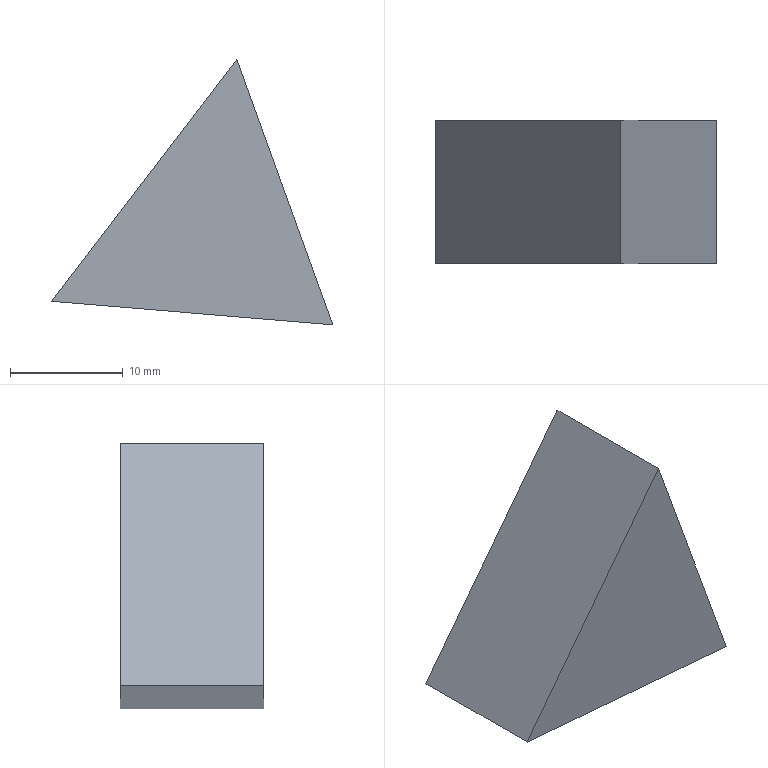Part | SolidWorks | features Extrusion 1 | 1 solid | 5 faces | box 24.913 x 12.7 x 23.516 mm | volume 3608 mm3 | plane 5
STEP:
#1=CARTESIAN_POINT('',(-8.486,0.,23.516));
#2=VERTEX_POINT('',#1);
#3=CARTESIAN_POINT('',(0.,0.,0.));
#4=VERTEX_POINT('',#3);
#5=CARTESIAN_POINT('',(-8.486,0.,23.516));
#6=DIRECTION('',(0.3395,0.,-0.9406));
#7=VECTOR('',#6,1000.);
#8=LINE('',#5,#7);
#9=EDGE_CURVE('',#2,#4,#8,.T.);
#10=ORIENTED_EDGE('',*,*,#9,.T.);
#11=CARTESIAN_POINT('',(0.,12.7,0.));
#12=VERTEX_POINT('',#11);
#13=CARTESIAN_POINT('',(0.,12.7,0.));
#14=DIRECTION('',(0.,-1.,0.));
#15=VECTOR('',#14,1000.);
#16=LINE('',#13,#15);
#17=EDGE_CURVE('',#12,#4,#16,.T.);
#18=ORIENTED_EDGE('',*,*,#17,.F.);
#19=CARTESIAN_POINT('',(-8.486,12.7,23.516));
#20=VERTEX_POINT('',#19);
#21=CARTESIAN_POINT('',(-8.486,12.7,23.516));
#22=DIRECTION('',(0.3395,0.,-0.9406));
#23=VECTOR('',#22,1000.);
#24=LINE('',#21,#23);
#25=EDGE_CURVE('',#20,#12,#24,.T.);
#26=ORIENTED_EDGE('',*,*,#25,.F.);
#27=CARTESIAN_POINT('',(-8.486,12.7,23.516));
#28=DIRECTION('',(0.,-1.,0.));
#29=VECTOR('',#28,1000.);
#30=LINE('',#27,#29);
#31=EDGE_CURVE('',#20,#2,#30,.T.);
#32=ORIENTED_EDGE('',*,*,#31,.T.);
#33=EDGE_LOOP('',(#10,#18,#26,#32));
#34=FACE_OUTER_BOUND('',#33,.T.);
#35=CARTESIAN_POINT('',(-8.486,12.7,23.516));
#36=DIRECTION('',(-0.9406,0.,-0.3395));
#37=DIRECTION('',(-0.3395,0.,0.9406));
#38=AXIS2_PLACEMENT_3D('',#35,#36,#37);
#39=PLANE('',#38);
#40=ADVANCED_FACE('',(#34),#39,.F.);
#41=CARTESIAN_POINT('',(-24.913,0.,2.087));
#42=VERTEX_POINT('',#41);
#43=CARTESIAN_POINT('',(0.,0.,0.));
#44=DIRECTION('',(-0.9965,0.,0.08349));
#45=VECTOR('',#44,1000.);
#46=LINE('',#43,#45);
#47=EDGE_CURVE('',#4,#42,#46,.T.);
#48=ORIENTED_EDGE('',*,*,#47,.T.);
#49=CARTESIAN_POINT('',(-24.913,12.7,2.087));
#50=VERTEX_POINT('',#49);
#51=CARTESIAN_POINT('',(-24.913,12.7,2.087));
#52=DIRECTION('',(0.,-1.,0.));
#53=VECTOR('',#52,1000.);
#54=LINE('',#51,#53);
#55=EDGE_CURVE('',#50,#42,#54,.T.);
#56=ORIENTED_EDGE('',*,*,#55,.F.);
#57=CARTESIAN_POINT('',(0.,12.7,0.));
#58=DIRECTION('',(-0.9965,0.,0.08349));
#59=VECTOR('',#58,1000.);
#60=LINE('',#57,#59);
#61=EDGE_CURVE('',#12,#50,#60,.T.);
#62=ORIENTED_EDGE('',*,*,#61,.F.);
#63=ORIENTED_EDGE('',*,*,#17,.T.);
#64=EDGE_LOOP('',(#48,#56,#62,#63));
#65=FACE_OUTER_BOUND('',#64,.T.);
#66=CARTESIAN_POINT('',(0.,12.7,0.));
#67=DIRECTION('',(0.08349,0.,0.9965));
#68=DIRECTION('',(0.9965,0.,-0.08349));
#69=AXIS2_PLACEMENT_3D('',#66,#67,#68);
#70=PLANE('',#69);
#71=ADVANCED_FACE('',(#65),#70,.F.);
#72=CARTESIAN_POINT('',(-24.913,0.,2.087));
#73=DIRECTION('',(0.6084,0.,0.7936));
#74=VECTOR('',#73,1000.);
#75=LINE('',#72,#74);
#76=EDGE_CURVE('',#42,#2,#75,.T.);
#77=ORIENTED_EDGE('',*,*,#76,.T.);
#78=ORIENTED_EDGE('',*,*,#31,.F.);
#79=CARTESIAN_POINT('',(-24.913,12.7,2.087));
#80=DIRECTION('',(0.6084,0.,0.7936));
#81=VECTOR('',#80,1000.);
#82=LINE('',#79,#81);
#83=EDGE_CURVE('',#50,#20,#82,.T.);
#84=ORIENTED_EDGE('',*,*,#83,.F.);
#85=ORIENTED_EDGE('',*,*,#55,.T.);
#86=EDGE_LOOP('',(#77,#78,#84,#85));
#87=FACE_OUTER_BOUND('',#86,.T.);
#88=CARTESIAN_POINT('',(-24.913,12.7,2.087));
#89=DIRECTION('',(0.7936,0.,-0.6084));
#90=DIRECTION('',(-0.6084,0.,-0.7936));
#91=AXIS2_PLACEMENT_3D('',#88,#89,#90);
#92=PLANE('',#91);
#93=ADVANCED_FACE('',(#87),#92,.F.);
#94=ORIENTED_EDGE('',*,*,#25,.T.);
#95=ORIENTED_EDGE('',*,*,#61,.T.);
#96=ORIENTED_EDGE('',*,*,#83,.T.);
#97=EDGE_LOOP('',(#94,#95,#96));
#98=FACE_OUTER_BOUND('',#97,.T.);
#99=CARTESIAN_POINT('',(0.,12.7,0.));
#100=DIRECTION('',(0.,1.,0.));
#101=DIRECTION('',(0.,0.,1.));
#102=AXIS2_PLACEMENT_3D('',#99,#100,#101);
#103=PLANE('',#102);
#104=ADVANCED_FACE('',(#98),#103,.T.);
#105=ORIENTED_EDGE('',*,*,#9,.F.);
#106=ORIENTED_EDGE('',*,*,#76,.F.);
#107=ORIENTED_EDGE('',*,*,#47,.F.);
#108=EDGE_LOOP('',(#105,#106,#107));
#109=FACE_OUTER_BOUND('',#108,.T.);
#110=CARTESIAN_POINT('',(0.,0.,0.));
#111=DIRECTION('',(0.,1.,0.));
#112=DIRECTION('',(0.,0.,1.));
#113=AXIS2_PLACEMENT_3D('',#110,#111,#112);
#114=PLANE('',#113);
#115=ADVANCED_FACE('',(#109),#114,.F.);
#116=CLOSED_SHELL('',(#40,#71,#93,#104,#115));
#117=MANIFOLD_SOLID_BREP('',#116);
#118=CARTESIAN_POINT('',(0.,0.,0.));
#119=DIRECTION('',(0.,0.,1.));
#120=DIRECTION('',(1.,0.,0.));
#121=AXIS2_PLACEMENT_3D('',#118,#119,#120);
#122=(LENGTH_UNIT()NAMED_UNIT(*)SI_UNIT(.MILLI.,.METRE.));
#123=UNCERTAINTY_MEASURE_WITH_UNIT(LENGTH_MEASURE(0.00001),#122,'','');
#124=(NAMED_UNIT(*)PLANE_ANGLE_UNIT()SI_UNIT($,.RADIAN.));
#125=(NAMED_UNIT(*)SI_UNIT($,.STERADIAN.)SOLID_ANGLE_UNIT());
#126=(GEOMETRIC_REPRESENTATION_CONTEXT(3)GLOBAL_UNCERTAINTY_ASSIGNED_CONTEXT((#123))GLOBAL_UNIT_ASSIGNED_CONTEXT((#122,#124,#125))REPRESENTATION_CONTEXT('',''));
#127=ADVANCED_BREP_SHAPE_REPRESENTATION('',(#117,#121),#126);